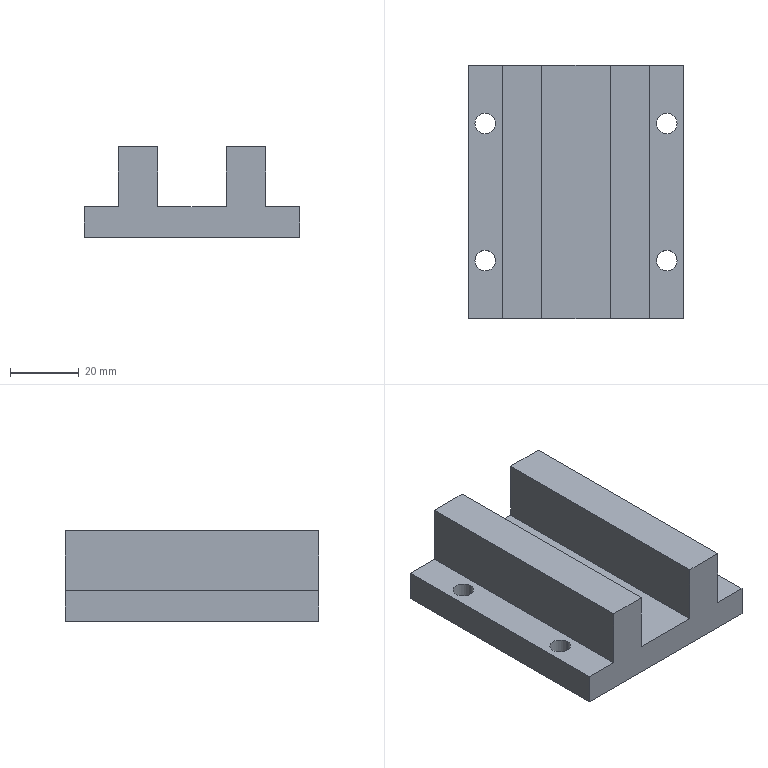Part | STEP file | Guide rail sliding pair | 1 solid | 22 faces | box 63 x 74 x 26.5 mm | volume 70725 mm3 | plane 14 | cylinder 8 | commonest cylinder face diameters 6 x8
STEP:
#1=CARTESIAN_POINT('',(9.179,-38.565,9.));
#2=VERTEX_POINT('',#1);
#3=CARTESIAN_POINT('',(3.179,-38.565,9.));
#4=VERTEX_POINT('',#3);
#5=CARTESIAN_POINT('',(6.179,-38.565,9.));
#6=DIRECTION('',(0.,0.,-1.));
#7=DIRECTION('',(-1.,0.,0.));
#8=AXIS2_PLACEMENT_3D('',#5,#6,#7);
#9=CIRCLE('',#8,3.);
#10=EDGE_CURVE('',#2,#4,#9,.T.);
#11=ORIENTED_EDGE('',*,*,#10,.F.);
#12=CARTESIAN_POINT('',(9.179,-38.565,0.));
#13=VERTEX_POINT('',#12);
#14=CARTESIAN_POINT('',(9.179,-38.565,9.));
#15=DIRECTION('',(0.,0.,-1.));
#16=VECTOR('',#15,1000.);
#17=LINE('',#14,#16);
#18=EDGE_CURVE('',#2,#13,#17,.T.);
#19=ORIENTED_EDGE('',*,*,#18,.T.);
#20=CARTESIAN_POINT('',(3.179,-38.565,0.));
#21=VERTEX_POINT('',#20);
#22=CARTESIAN_POINT('',(6.179,-38.565,0.));
#23=DIRECTION('',(0.,0.,-1.));
#24=DIRECTION('',(-1.,0.,0.));
#25=AXIS2_PLACEMENT_3D('',#22,#23,#24);
#26=CIRCLE('',#25,3.);
#27=EDGE_CURVE('',#13,#21,#26,.T.);
#28=ORIENTED_EDGE('',*,*,#27,.T.);
#29=CARTESIAN_POINT('',(3.179,-38.565,9.));
#30=DIRECTION('',(0.,0.,-1.));
#31=VECTOR('',#30,1000.);
#32=LINE('',#29,#31);
#33=EDGE_CURVE('',#4,#21,#32,.T.);
#34=ORIENTED_EDGE('',*,*,#33,.F.);
#35=EDGE_LOOP('',(#11,#19,#28,#34));
#36=FACE_OUTER_BOUND('',#35,.T.);
#37=CARTESIAN_POINT('',(6.179,-38.565,9.));
#38=DIRECTION('',(0.,0.,-1.));
#39=DIRECTION('',(-1.,0.,0.));
#40=AXIS2_PLACEMENT_3D('',#37,#38,#39);
#41=CYLINDRICAL_SURFACE('',#40,3.);
#42=ADVANCED_FACE('',(#36),#41,.F.);
#43=CARTESIAN_POINT('',(9.179,1.435,9.));
#44=VERTEX_POINT('',#43);
#45=CARTESIAN_POINT('',(3.179,1.435,9.));
#46=VERTEX_POINT('',#45);
#47=CARTESIAN_POINT('',(6.179,1.435,9.));
#48=DIRECTION('',(0.,0.,-1.));
#49=DIRECTION('',(-1.,0.,0.));
#50=AXIS2_PLACEMENT_3D('',#47,#48,#49);
#51=CIRCLE('',#50,3.);
#52=EDGE_CURVE('',#44,#46,#51,.T.);
#53=ORIENTED_EDGE('',*,*,#52,.F.);
#54=CARTESIAN_POINT('',(9.179,1.435,0.));
#55=VERTEX_POINT('',#54);
#56=CARTESIAN_POINT('',(9.179,1.435,9.));
#57=DIRECTION('',(0.,0.,-1.));
#58=VECTOR('',#57,1000.);
#59=LINE('',#56,#58);
#60=EDGE_CURVE('',#44,#55,#59,.T.);
#61=ORIENTED_EDGE('',*,*,#60,.T.);
#62=CARTESIAN_POINT('',(3.179,1.435,0.));
#63=VERTEX_POINT('',#62);
#64=CARTESIAN_POINT('',(6.179,1.435,0.));
#65=DIRECTION('',(0.,0.,-1.));
#66=DIRECTION('',(-1.,0.,0.));
#67=AXIS2_PLACEMENT_3D('',#64,#65,#66);
#68=CIRCLE('',#67,3.);
#69=EDGE_CURVE('',#55,#63,#68,.T.);
#70=ORIENTED_EDGE('',*,*,#69,.T.);
#71=CARTESIAN_POINT('',(3.179,1.435,9.));
#72=DIRECTION('',(0.,0.,-1.));
#73=VECTOR('',#72,1000.);
#74=LINE('',#71,#73);
#75=EDGE_CURVE('',#46,#63,#74,.T.);
#76=ORIENTED_EDGE('',*,*,#75,.F.);
#77=EDGE_LOOP('',(#53,#61,#70,#76));
#78=FACE_OUTER_BOUND('',#77,.T.);
#79=CARTESIAN_POINT('',(6.179,1.435,9.));
#80=DIRECTION('',(0.,0.,-1.));
#81=DIRECTION('',(-1.,0.,0.));
#82=AXIS2_PLACEMENT_3D('',#79,#80,#81);
#83=CYLINDRICAL_SURFACE('',#82,3.);
#84=ADVANCED_FACE('',(#78),#83,.F.);
#85=CARTESIAN_POINT('',(-43.821,1.435,9.));
#86=VERTEX_POINT('',#85);
#87=CARTESIAN_POINT('',(-49.821,1.435,9.));
#88=VERTEX_POINT('',#87);
#89=CARTESIAN_POINT('',(-46.821,1.435,9.));
#90=DIRECTION('',(0.,0.,-1.));
#91=DIRECTION('',(-1.,0.,0.));
#92=AXIS2_PLACEMENT_3D('',#89,#90,#91);
#93=CIRCLE('',#92,3.);
#94=EDGE_CURVE('',#86,#88,#93,.T.);
#95=ORIENTED_EDGE('',*,*,#94,.F.);
#96=CARTESIAN_POINT('',(-43.821,1.435,0.));
#97=VERTEX_POINT('',#96);
#98=CARTESIAN_POINT('',(-43.821,1.435,9.));
#99=DIRECTION('',(0.,0.,-1.));
#100=VECTOR('',#99,1000.);
#101=LINE('',#98,#100);
#102=EDGE_CURVE('',#86,#97,#101,.T.);
#103=ORIENTED_EDGE('',*,*,#102,.T.);
#104=CARTESIAN_POINT('',(-49.821,1.435,0.));
#105=VERTEX_POINT('',#104);
#106=CARTESIAN_POINT('',(-46.821,1.435,0.));
#107=DIRECTION('',(0.,0.,-1.));
#108=DIRECTION('',(-1.,0.,0.));
#109=AXIS2_PLACEMENT_3D('',#106,#107,#108);
#110=CIRCLE('',#109,3.);
#111=EDGE_CURVE('',#97,#105,#110,.T.);
#112=ORIENTED_EDGE('',*,*,#111,.T.);
#113=CARTESIAN_POINT('',(-49.821,1.435,9.));
#114=DIRECTION('',(0.,0.,-1.));
#115=VECTOR('',#114,1000.);
#116=LINE('',#113,#115);
#117=EDGE_CURVE('',#88,#105,#116,.T.);
#118=ORIENTED_EDGE('',*,*,#117,.F.);
#119=EDGE_LOOP('',(#95,#103,#112,#118));
#120=FACE_OUTER_BOUND('',#119,.T.);
#121=CARTESIAN_POINT('',(-46.821,1.435,9.));
#122=DIRECTION('',(0.,0.,-1.));
#123=DIRECTION('',(-1.,0.,0.));
#124=AXIS2_PLACEMENT_3D('',#121,#122,#123);
#125=CYLINDRICAL_SURFACE('',#124,3.);
#126=ADVANCED_FACE('',(#120),#125,.F.);
#127=CARTESIAN_POINT('',(-43.821,-38.565,9.));
#128=VERTEX_POINT('',#127);
#129=CARTESIAN_POINT('',(-49.821,-38.565,9.));
#130=VERTEX_POINT('',#129);
#131=CARTESIAN_POINT('',(-46.821,-38.565,9.));
#132=DIRECTION('',(0.,0.,-1.));
#133=DIRECTION('',(-1.,0.,0.));
#134=AXIS2_PLACEMENT_3D('',#131,#132,#133);
#135=CIRCLE('',#134,3.);
#136=EDGE_CURVE('',#128,#130,#135,.T.);
#137=ORIENTED_EDGE('',*,*,#136,.F.);
#138=CARTESIAN_POINT('',(-43.821,-38.565,0.));
#139=VERTEX_POINT('',#138);
#140=CARTESIAN_POINT('',(-43.821,-38.565,9.));
#141=DIRECTION('',(0.,0.,-1.));
#142=VECTOR('',#141,1000.);
#143=LINE('',#140,#142);
#144=EDGE_CURVE('',#128,#139,#143,.T.);
#145=ORIENTED_EDGE('',*,*,#144,.T.);
#146=CARTESIAN_POINT('',(-49.821,-38.565,0.));
#147=VERTEX_POINT('',#146);
#148=CARTESIAN_POINT('',(-46.821,-38.565,0.));
#149=DIRECTION('',(0.,0.,-1.));
#150=DIRECTION('',(-1.,0.,0.));
#151=AXIS2_PLACEMENT_3D('',#148,#149,#150);
#152=CIRCLE('',#151,3.);
#153=EDGE_CURVE('',#139,#147,#152,.T.);
#154=ORIENTED_EDGE('',*,*,#153,.T.);
#155=CARTESIAN_POINT('',(-49.821,-38.565,9.));
#156=DIRECTION('',(0.,0.,-1.));
#157=VECTOR('',#156,1000.);
#158=LINE('',#155,#157);
#159=EDGE_CURVE('',#130,#147,#158,.T.);
#160=ORIENTED_EDGE('',*,*,#159,.F.);
#161=EDGE_LOOP('',(#137,#145,#154,#160));
#162=FACE_OUTER_BOUND('',#161,.T.);
#163=CARTESIAN_POINT('',(-46.821,-38.565,9.));
#164=DIRECTION('',(0.,0.,-1.));
#165=DIRECTION('',(-1.,0.,0.));
#166=AXIS2_PLACEMENT_3D('',#163,#164,#165);
#167=CYLINDRICAL_SURFACE('',#166,3.);
#168=ADVANCED_FACE('',(#162),#167,.F.);
#169=CARTESIAN_POINT('',(6.179,-38.565,0.));
#170=DIRECTION('',(0.,0.,-1.));
#171=DIRECTION('',(-1.,0.,0.));
#172=AXIS2_PLACEMENT_3D('',#169,#170,#171);
#173=CIRCLE('',#172,3.);
#174=EDGE_CURVE('',#21,#13,#173,.T.);
#175=ORIENTED_EDGE('',*,*,#174,.F.);
#176=ORIENTED_EDGE('',*,*,#27,.F.);
#177=EDGE_LOOP('',(#175,#176));
#178=FACE_BOUND('',#177,.T.);
#179=CARTESIAN_POINT('',(6.179,1.435,0.));
#180=DIRECTION('',(0.,0.,-1.));
#181=DIRECTION('',(-1.,0.,0.));
#182=AXIS2_PLACEMENT_3D('',#179,#180,#181);
#183=CIRCLE('',#182,3.);
#184=EDGE_CURVE('',#63,#55,#183,.T.);
#185=ORIENTED_EDGE('',*,*,#184,.F.);
#186=ORIENTED_EDGE('',*,*,#69,.F.);
#187=EDGE_LOOP('',(#185,#186));
#188=FACE_BOUND('',#187,.T.);
#189=CARTESIAN_POINT('',(11.179,18.435,0.));
#190=VERTEX_POINT('',#189);
#191=CARTESIAN_POINT('',(-51.821,18.435,0.));
#192=VERTEX_POINT('',#191);
#193=CARTESIAN_POINT('',(-51.821,18.435,0.));
#194=DIRECTION('',(-1.,0.,0.));
#195=VECTOR('',#194,1000.);
#196=LINE('',#193,#195);
#197=EDGE_CURVE('',#190,#192,#196,.T.);
#198=ORIENTED_EDGE('',*,*,#197,.F.);
#199=CARTESIAN_POINT('',(11.179,-55.565,0.));
#200=VERTEX_POINT('',#199);
#201=CARTESIAN_POINT('',(11.179,-55.565,0.));
#202=DIRECTION('',(0.,1.,0.));
#203=VECTOR('',#202,1000.);
#204=LINE('',#201,#203);
#205=EDGE_CURVE('',#200,#190,#204,.T.);
#206=ORIENTED_EDGE('',*,*,#205,.F.);
#207=CARTESIAN_POINT('',(-51.821,-55.565,0.));
#208=VERTEX_POINT('',#207);
#209=CARTESIAN_POINT('',(-51.821,-55.565,0.));
#210=DIRECTION('',(1.,0.,0.));
#211=VECTOR('',#210,1000.);
#212=LINE('',#209,#211);
#213=EDGE_CURVE('',#208,#200,#212,.T.);
#214=ORIENTED_EDGE('',*,*,#213,.F.);
#215=CARTESIAN_POINT('',(-51.821,-55.565,0.));
#216=DIRECTION('',(0.,-1.,0.));
#217=VECTOR('',#216,1000.);
#218=LINE('',#215,#217);
#219=EDGE_CURVE('',#192,#208,#218,.T.);
#220=ORIENTED_EDGE('',*,*,#219,.F.);
#221=EDGE_LOOP('',(#198,#206,#214,#220));
#222=FACE_OUTER_BOUND('',#221,.T.);
#223=CARTESIAN_POINT('',(-46.821,1.435,0.));
#224=DIRECTION('',(0.,0.,-1.));
#225=DIRECTION('',(-1.,0.,0.));
#226=AXIS2_PLACEMENT_3D('',#223,#224,#225);
#227=CIRCLE('',#226,3.);
#228=EDGE_CURVE('',#105,#97,#227,.T.);
#229=ORIENTED_EDGE('',*,*,#228,.F.);
#230=ORIENTED_EDGE('',*,*,#111,.F.);
#231=EDGE_LOOP('',(#229,#230));
#232=FACE_BOUND('',#231,.T.);
#233=CARTESIAN_POINT('',(-46.821,-38.565,0.));
#234=DIRECTION('',(0.,0.,-1.));
#235=DIRECTION('',(-1.,0.,0.));
#236=AXIS2_PLACEMENT_3D('',#233,#234,#235);
#237=CIRCLE('',#236,3.);
#238=EDGE_CURVE('',#147,#139,#237,.T.);
#239=ORIENTED_EDGE('',*,*,#238,.F.);
#240=ORIENTED_EDGE('',*,*,#153,.F.);
#241=EDGE_LOOP('',(#239,#240));
#242=FACE_BOUND('',#241,.T.);
#243=CARTESIAN_POINT('',(-51.821,-55.565,0.));
#244=DIRECTION('',(0.,0.,1.));
#245=DIRECTION('',(1.,0.,0.));
#246=AXIS2_PLACEMENT_3D('',#243,#244,#245);
#247=PLANE('',#246);
#248=ADVANCED_FACE('',(#178,#188,#222,#232,#242),#247,.F.);
#249=ORIENTED_EDGE('',*,*,#18,.F.);
#250=CARTESIAN_POINT('',(6.179,-38.565,9.));
#251=DIRECTION('',(0.,0.,-1.));
#252=DIRECTION('',(-1.,0.,0.));
#253=AXIS2_PLACEMENT_3D('',#250,#251,#252);
#254=CIRCLE('',#253,3.);
#255=EDGE_CURVE('',#4,#2,#254,.T.);
#256=ORIENTED_EDGE('',*,*,#255,.F.);
#257=ORIENTED_EDGE('',*,*,#33,.T.);
#258=ORIENTED_EDGE('',*,*,#174,.T.);
#259=EDGE_LOOP('',(#249,#256,#257,#258));
#260=FACE_OUTER_BOUND('',#259,.T.);
#261=CARTESIAN_POINT('',(6.179,-38.565,9.));
#262=DIRECTION('',(0.,0.,-1.));
#263=DIRECTION('',(-1.,0.,0.));
#264=AXIS2_PLACEMENT_3D('',#261,#262,#263);
#265=CYLINDRICAL_SURFACE('',#264,3.);
#266=ADVANCED_FACE('',(#260),#265,.F.);
#267=ORIENTED_EDGE('',*,*,#60,.F.);
#268=CARTESIAN_POINT('',(6.179,1.435,9.));
#269=DIRECTION('',(0.,0.,-1.));
#270=DIRECTION('',(-1.,0.,0.));
#271=AXIS2_PLACEMENT_3D('',#268,#269,#270);
#272=CIRCLE('',#271,3.);
#273=EDGE_CURVE('',#46,#44,#272,.T.);
#274=ORIENTED_EDGE('',*,*,#273,.F.);
#275=ORIENTED_EDGE('',*,*,#75,.T.);
#276=ORIENTED_EDGE('',*,*,#184,.T.);
#277=EDGE_LOOP('',(#267,#274,#275,#276));
#278=FACE_OUTER_BOUND('',#277,.T.);
#279=CARTESIAN_POINT('',(6.179,1.435,9.));
#280=DIRECTION('',(0.,0.,-1.));
#281=DIRECTION('',(-1.,0.,0.));
#282=AXIS2_PLACEMENT_3D('',#279,#280,#281);
#283=CYLINDRICAL_SURFACE('',#282,3.);
#284=ADVANCED_FACE('',(#278),#283,.F.);
#285=CARTESIAN_POINT('',(-51.821,-55.565,9.));
#286=VERTEX_POINT('',#285);
#287=CARTESIAN_POINT('',(-51.821,-55.565,9.));
#288=DIRECTION('',(0.,0.,-1.));
#289=VECTOR('',#288,1000.);
#290=LINE('',#287,#289);
#291=EDGE_CURVE('',#286,#208,#290,.T.);
#292=ORIENTED_EDGE('',*,*,#291,.F.);
#293=CARTESIAN_POINT('',(-51.821,18.435,9.));
#294=VERTEX_POINT('',#293);
#295=CARTESIAN_POINT('',(-51.821,18.435,9.));
#296=DIRECTION('',(0.,-1.,0.));
#297=VECTOR('',#296,1000.);
#298=LINE('',#295,#297);
#299=EDGE_CURVE('',#294,#286,#298,.T.);
#300=ORIENTED_EDGE('',*,*,#299,.F.);
#301=CARTESIAN_POINT('',(-51.821,18.435,9.));
#302=DIRECTION('',(0.,0.,1.));
#303=VECTOR('',#302,1000.);
#304=LINE('',#301,#303);
#305=EDGE_CURVE('',#192,#294,#304,.T.);
#306=ORIENTED_EDGE('',*,*,#305,.F.);
#307=ORIENTED_EDGE('',*,*,#219,.T.);
#308=EDGE_LOOP('',(#292,#300,#306,#307));
#309=FACE_OUTER_BOUND('',#308,.T.);
#310=CARTESIAN_POINT('',(-51.821,18.435,9.));
#311=DIRECTION('',(1.,0.,0.));
#312=DIRECTION('',(0.,0.,-1.));
#313=AXIS2_PLACEMENT_3D('',#310,#311,#312);
#314=PLANE('',#313);
#315=ADVANCED_FACE('',(#309),#314,.F.);
#316=CARTESIAN_POINT('',(-30.321,18.435,9.));
#317=VERTEX_POINT('',#316);
#318=CARTESIAN_POINT('',(-30.321,18.435,26.5));
#319=VERTEX_POINT('',#318);
#320=CARTESIAN_POINT('',(-30.321,18.435,9.));
#321=DIRECTION('',(0.,0.,1.));
#322=VECTOR('',#321,1000.);
#323=LINE('',#320,#322);
#324=EDGE_CURVE('',#317,#319,#323,.T.);
#325=ORIENTED_EDGE('',*,*,#324,.F.);
#326=CARTESIAN_POINT('',(-10.321,18.435,9.));
#327=VERTEX_POINT('',#326);
#328=CARTESIAN_POINT('',(-51.821,18.435,9.));
#329=DIRECTION('',(-1.,0.,0.));
#330=VECTOR('',#329,1000.);
#331=LINE('',#328,#330);
#332=EDGE_CURVE('',#327,#317,#331,.T.);
#333=ORIENTED_EDGE('',*,*,#332,.F.);
#334=CARTESIAN_POINT('',(-10.321,18.435,26.5));
#335=VERTEX_POINT('',#334);
#336=CARTESIAN_POINT('',(-10.321,18.435,9.));
#337=DIRECTION('',(0.,0.,-1.));
#338=VECTOR('',#337,1000.);
#339=LINE('',#336,#338);
#340=EDGE_CURVE('',#335,#327,#339,.T.);
#341=ORIENTED_EDGE('',*,*,#340,.F.);
#342=CARTESIAN_POINT('',(1.179,18.435,26.5));
#343=VERTEX_POINT('',#342);
#344=CARTESIAN_POINT('',(-51.821,18.435,26.5));
#345=DIRECTION('',(-1.,0.,0.));
#346=VECTOR('',#345,1000.);
#347=LINE('',#344,#346);
#348=EDGE_CURVE('',#343,#335,#347,.T.);
#349=ORIENTED_EDGE('',*,*,#348,.F.);
#350=CARTESIAN_POINT('',(1.179,18.435,9.));
#351=VERTEX_POINT('',#350);
#352=CARTESIAN_POINT('',(1.179,18.435,9.));
#353=DIRECTION('',(0.,0.,1.));
#354=VECTOR('',#353,1000.);
#355=LINE('',#352,#354);
#356=EDGE_CURVE('',#351,#343,#355,.T.);
#357=ORIENTED_EDGE('',*,*,#356,.F.);
#358=CARTESIAN_POINT('',(11.179,18.435,9.));
#359=VERTEX_POINT('',#358);
#360=CARTESIAN_POINT('',(-51.821,18.435,9.));
#361=DIRECTION('',(-1.,0.,0.));
#362=VECTOR('',#361,1000.);
#363=LINE('',#360,#362);
#364=EDGE_CURVE('',#359,#351,#363,.T.);
#365=ORIENTED_EDGE('',*,*,#364,.F.);
#366=CARTESIAN_POINT('',(11.179,18.435,9.));
#367=DIRECTION('',(0.,0.,1.));
#368=VECTOR('',#367,1000.);
#369=LINE('',#366,#368);
#370=EDGE_CURVE('',#190,#359,#369,.T.);
#371=ORIENTED_EDGE('',*,*,#370,.F.);
#372=ORIENTED_EDGE('',*,*,#197,.T.);
#373=ORIENTED_EDGE('',*,*,#305,.T.);
#374=CARTESIAN_POINT('',(-41.821,18.435,9.));
#375=VERTEX_POINT('',#374);
#376=CARTESIAN_POINT('',(-51.821,18.435,9.));
#377=DIRECTION('',(-1.,0.,0.));
#378=VECTOR('',#377,1000.);
#379=LINE('',#376,#378);
#380=EDGE_CURVE('',#375,#294,#379,.T.);
#381=ORIENTED_EDGE('',*,*,#380,.F.);
#382=CARTESIAN_POINT('',(-41.821,18.435,26.5));
#383=VERTEX_POINT('',#382);
#384=CARTESIAN_POINT('',(-41.821,18.435,9.));
#385=DIRECTION('',(0.,0.,-1.));
#386=VECTOR('',#385,1000.);
#387=LINE('',#384,#386);
#388=EDGE_CURVE('',#383,#375,#387,.T.);
#389=ORIENTED_EDGE('',*,*,#388,.F.);
#390=CARTESIAN_POINT('',(-51.821,18.435,26.5));
#391=DIRECTION('',(-1.,0.,0.));
#392=VECTOR('',#391,1000.);
#393=LINE('',#390,#392);
#394=EDGE_CURVE('',#319,#383,#393,.T.);
#395=ORIENTED_EDGE('',*,*,#394,.F.);
#396=EDGE_LOOP('',(#325,#333,#341,#349,#357,#365,#371,#372,#373,#381,#389,#395));
#397=FACE_OUTER_BOUND('',#396,.T.);
#398=CARTESIAN_POINT('',(-51.821,18.435,9.));
#399=DIRECTION('',(0.,-1.,0.));
#400=DIRECTION('',(0.,0.,-1.));
#401=AXIS2_PLACEMENT_3D('',#398,#399,#400);
#402=PLANE('',#401);
#403=ADVANCED_FACE('',(#397),#402,.F.);
#404=ORIENTED_EDGE('',*,*,#370,.T.);
#405=CARTESIAN_POINT('',(11.179,-55.565,9.));
#406=VERTEX_POINT('',#405);
#407=CARTESIAN_POINT('',(11.179,18.435,9.));
#408=DIRECTION('',(0.,1.,0.));
#409=VECTOR('',#408,1000.);
#410=LINE('',#407,#409);
#411=EDGE_CURVE('',#406,#359,#410,.T.);
#412=ORIENTED_EDGE('',*,*,#411,.F.);
#413=CARTESIAN_POINT('',(11.179,-55.565,9.));
#414=DIRECTION('',(0.,0.,1.));
#415=VECTOR('',#414,1000.);
#416=LINE('',#413,#415);
#417=EDGE_CURVE('',#200,#406,#416,.T.);
#418=ORIENTED_EDGE('',*,*,#417,.F.);
#419=ORIENTED_EDGE('',*,*,#205,.T.);
#420=EDGE_LOOP('',(#404,#412,#418,#419));
#421=FACE_OUTER_BOUND('',#420,.T.);
#422=CARTESIAN_POINT('',(11.179,18.435,9.));
#423=DIRECTION('',(-1.,0.,0.));
#424=DIRECTION('',(0.,0.,1.));
#425=AXIS2_PLACEMENT_3D('',#422,#423,#424);
#426=PLANE('',#425);
#427=ADVANCED_FACE('',(#421),#426,.F.);
#428=CARTESIAN_POINT('',(-30.321,-55.565,26.5));
#429=VERTEX_POINT('',#428);
#430=CARTESIAN_POINT('',(-30.321,-55.565,9.));
#431=VERTEX_POINT('',#430);
#432=CARTESIAN_POINT('',(-30.321,-55.565,9.));
#433=DIRECTION('',(0.,0.,-1.));
#434=VECTOR('',#433,1000.);
#435=LINE('',#432,#434);
#436=EDGE_CURVE('',#429,#431,#435,.T.);
#437=ORIENTED_EDGE('',*,*,#436,.F.);
#438=CARTESIAN_POINT('',(-41.821,-55.565,26.5));
#439=VERTEX_POINT('',#438);
#440=CARTESIAN_POINT('',(-51.821,-55.565,26.5));
#441=DIRECTION('',(1.,0.,0.));
#442=VECTOR('',#441,1000.);
#443=LINE('',#440,#442);
#444=EDGE_CURVE('',#439,#429,#443,.T.);
#445=ORIENTED_EDGE('',*,*,#444,.F.);
#446=CARTESIAN_POINT('',(-41.821,-55.565,9.));
#447=VERTEX_POINT('',#446);
#448=CARTESIAN_POINT('',(-41.821,-55.565,9.));
#449=DIRECTION('',(0.,0.,1.));
#450=VECTOR('',#449,1000.);
#451=LINE('',#448,#450);
#452=EDGE_CURVE('',#447,#439,#451,.T.);
#453=ORIENTED_EDGE('',*,*,#452,.F.);
#454=CARTESIAN_POINT('',(-51.821,-55.565,9.));
#455=DIRECTION('',(1.,0.,0.));
#456=VECTOR('',#455,1000.);
#457=LINE('',#454,#456);
#458=EDGE_CURVE('',#286,#447,#457,.T.);
#459=ORIENTED_EDGE('',*,*,#458,.F.);
#460=ORIENTED_EDGE('',*,*,#291,.T.);
#461=ORIENTED_EDGE('',*,*,#213,.T.);
#462=ORIENTED_EDGE('',*,*,#417,.T.);
#463=CARTESIAN_POINT('',(1.179,-55.565,9.));
#464=VERTEX_POINT('',#463);
#465=CARTESIAN_POINT('',(-51.821,-55.565,9.));
#466=DIRECTION('',(1.,0.,0.));
#467=VECTOR('',#466,1000.);
#468=LINE('',#465,#467);
#469=EDGE_CURVE('',#464,#406,#468,.T.);
#470=ORIENTED_EDGE('',*,*,#469,.F.);
#471=CARTESIAN_POINT('',(1.179,-55.565,26.5));
#472=VERTEX_POINT('',#471);
#473=CARTESIAN_POINT('',(1.179,-55.565,9.));
#474=DIRECTION('',(0.,0.,-1.));
#475=VECTOR('',#474,1000.);
#476=LINE('',#473,#475);
#477=EDGE_CURVE('',#472,#464,#476,.T.);
#478=ORIENTED_EDGE('',*,*,#477,.F.);
#479=CARTESIAN_POINT('',(-10.321,-55.565,26.5));
#480=VERTEX_POINT('',#479);
#481=CARTESIAN_POINT('',(-51.821,-55.565,26.5));
#482=DIRECTION('',(1.,0.,0.));
#483=VECTOR('',#482,1000.);
#484=LINE('',#481,#483);
#485=EDGE_CURVE('',#480,#472,#484,.T.);
#486=ORIENTED_EDGE('',*,*,#485,.F.);
#487=CARTESIAN_POINT('',(-10.321,-55.565,9.));
#488=VERTEX_POINT('',#487);
#489=CARTESIAN_POINT('',(-10.321,-55.565,9.));
#490=DIRECTION('',(0.,0.,1.));
#491=VECTOR('',#490,1000.);
#492=LINE('',#489,#491);
#493=EDGE_CURVE('',#488,#480,#492,.T.);
#494=ORIENTED_EDGE('',*,*,#493,.F.);
#495=CARTESIAN_POINT('',(-51.821,-55.565,9.));
#496=DIRECTION('',(1.,0.,0.));
#497=VECTOR('',#496,1000.);
#498=LINE('',#495,#497);
#499=EDGE_CURVE('',#431,#488,#498,.T.);
#500=ORIENTED_EDGE('',*,*,#499,.F.);
#501=EDGE_LOOP('',(#437,#445,#453,#459,#460,#461,#462,#470,#478,#486,#494,#500));
#502=FACE_OUTER_BOUND('',#501,.T.);
#503=CARTESIAN_POINT('',(-51.821,-55.565,9.));
#504=DIRECTION('',(0.,1.,0.));
#505=DIRECTION('',(0.,0.,1.));
#506=AXIS2_PLACEMENT_3D('',#503,#504,#505);
#507=PLANE('',#506);
#508=ADVANCED_FACE('',(#502),#507,.F.);
#509=ORIENTED_EDGE('',*,*,#102,.F.);
#510=CARTESIAN_POINT('',(-46.821,1.435,9.));
#511=DIRECTION('',(0.,0.,-1.));
#512=DIRECTION('',(-1.,0.,0.));
#513=AXIS2_PLACEMENT_3D('',#510,#511,#512);
#514=CIRCLE('',#513,3.);
#515=EDGE_CURVE('',#88,#86,#514,.T.);
#516=ORIENTED_EDGE('',*,*,#515,.F.);
#517=ORIENTED_EDGE('',*,*,#117,.T.);
#518=ORIENTED_EDGE('',*,*,#228,.T.);
#519=EDGE_LOOP('',(#509,#516,#517,#518));
#520=FACE_OUTER_BOUND('',#519,.T.);
#521=CARTESIAN_POINT('',(-46.821,1.435,9.));
#522=DIRECTION('',(0.,0.,-1.));
#523=DIRECTION('',(-1.,0.,0.));
#524=AXIS2_PLACEMENT_3D('',#521,#522,#523);
#525=CYLINDRICAL_SURFACE('',#524,3.);
#526=ADVANCED_FACE('',(#520),#525,.F.);
#527=ORIENTED_EDGE('',*,*,#144,.F.);
#528=CARTESIAN_POINT('',(-46.821,-38.565,9.));
#529=DIRECTION('',(0.,0.,-1.));
#530=DIRECTION('',(-1.,0.,0.));
#531=AXIS2_PLACEMENT_3D('',#528,#529,#530);
#532=CIRCLE('',#531,3.);
#533=EDGE_CURVE('',#130,#128,#532,.T.);
#534=ORIENTED_EDGE('',*,*,#533,.F.);
#535=ORIENTED_EDGE('',*,*,#159,.T.);
#536=ORIENTED_EDGE('',*,*,#238,.T.);
#537=EDGE_LOOP('',(#527,#534,#535,#536));
#538=FACE_OUTER_BOUND('',#537,.T.);
#539=CARTESIAN_POINT('',(-46.821,-38.565,9.));
#540=DIRECTION('',(0.,0.,-1.));
#541=DIRECTION('',(-1.,0.,0.));
#542=AXIS2_PLACEMENT_3D('',#539,#540,#541);
#543=CYLINDRICAL_SURFACE('',#542,3.);
#544=ADVANCED_FACE('',(#538),#543,.F.);
#545=ORIENTED_EDGE('',*,*,#255,.T.);
#546=ORIENTED_EDGE('',*,*,#10,.T.);
#547=EDGE_LOOP('',(#545,#546));
#548=FACE_BOUND('',#547,.T.);
#549=ORIENTED_EDGE('',*,*,#273,.T.);
#550=ORIENTED_EDGE('',*,*,#52,.T.);
#551=EDGE_LOOP('',(#549,#550));
#552=FACE_BOUND('',#551,.T.);
#553=ORIENTED_EDGE('',*,*,#411,.T.);
#554=ORIENTED_EDGE('',*,*,#364,.T.);
#555=CARTESIAN_POINT('',(1.179,-55.565,9.));
#556=DIRECTION('',(0.,-1.,0.));
#557=VECTOR('',#556,1000.);
#558=LINE('',#555,#557);
#559=EDGE_CURVE('',#351,#464,#558,.T.);
#560=ORIENTED_EDGE('',*,*,#559,.T.);
#561=ORIENTED_EDGE('',*,*,#469,.T.);
#562=EDGE_LOOP('',(#553,#554,#560,#561));
#563=FACE_OUTER_BOUND('',#562,.T.);
#564=CARTESIAN_POINT('',(-51.821,-55.565,9.));
#565=DIRECTION('',(0.,0.,1.));
#566=DIRECTION('',(1.,0.,0.));
#567=AXIS2_PLACEMENT_3D('',#564,#565,#566);
#568=PLANE('',#567);
#569=ADVANCED_FACE('',(#548,#552,#563),#568,.T.);
#570=ORIENTED_EDGE('',*,*,#533,.T.);
#571=ORIENTED_EDGE('',*,*,#136,.T.);
#572=EDGE_LOOP('',(#570,#571));
#573=FACE_BOUND('',#572,.T.);
#574=ORIENTED_EDGE('',*,*,#515,.T.);
#575=ORIENTED_EDGE('',*,*,#94,.T.);
#576=EDGE_LOOP('',(#574,#575));
#577=FACE_BOUND('',#576,.T.);
#578=ORIENTED_EDGE('',*,*,#299,.T.);
#579=ORIENTED_EDGE('',*,*,#458,.T.);
#580=CARTESIAN_POINT('',(-41.821,-55.565,9.));
#581=DIRECTION('',(0.,1.,0.));
#582=VECTOR('',#581,1000.);
#583=LINE('',#580,#582);
#584=EDGE_CURVE('',#447,#375,#583,.T.);
#585=ORIENTED_EDGE('',*,*,#584,.T.);
#586=ORIENTED_EDGE('',*,*,#380,.T.);
#587=EDGE_LOOP('',(#578,#579,#585,#586));
#588=FACE_OUTER_BOUND('',#587,.T.);
#589=CARTESIAN_POINT('',(-51.821,-55.565,9.));
#590=DIRECTION('',(0.,0.,1.));
#591=DIRECTION('',(1.,0.,0.));
#592=AXIS2_PLACEMENT_3D('',#589,#590,#591);
#593=PLANE('',#592);
#594=ADVANCED_FACE('',(#573,#577,#588),#593,.T.);
#595=CARTESIAN_POINT('',(-41.821,-55.565,26.5));
#596=DIRECTION('',(0.,-1.,0.));
#597=VECTOR('',#596,1000.);
#598=LINE('',#595,#597);
#599=EDGE_CURVE('',#383,#439,#598,.T.);
#600=ORIENTED_EDGE('',*,*,#599,.T.);
#601=ORIENTED_EDGE('',*,*,#444,.T.);
#602=CARTESIAN_POINT('',(-30.321,-55.565,26.5));
#603=DIRECTION('',(0.,1.,0.));
#604=VECTOR('',#603,1000.);
#605=LINE('',#602,#604);
#606=EDGE_CURVE('',#429,#319,#605,.T.);
#607=ORIENTED_EDGE('',*,*,#606,.T.);
#608=ORIENTED_EDGE('',*,*,#394,.T.);
#609=EDGE_LOOP('',(#600,#601,#607,#608));
#610=FACE_OUTER_BOUND('',#609,.T.);
#611=CARTESIAN_POINT('',(-41.821,-55.565,26.5));
#612=DIRECTION('',(0.,0.,1.));
#613=DIRECTION('',(1.,0.,0.));
#614=AXIS2_PLACEMENT_3D('',#611,#612,#613);
#615=PLANE('',#614);
#616=ADVANCED_FACE('',(#610),#615,.T.);
#617=ORIENTED_EDGE('',*,*,#436,.T.);
#618=CARTESIAN_POINT('',(-30.321,18.435,9.));
#619=DIRECTION('',(0.,-1.,0.));
#620=VECTOR('',#619,1000.);
#621=LINE('',#618,#620);
#622=EDGE_CURVE('',#317,#431,#621,.T.);
#623=ORIENTED_EDGE('',*,*,#622,.F.);
#624=ORIENTED_EDGE('',*,*,#324,.T.);
#625=ORIENTED_EDGE('',*,*,#606,.F.);
#626=EDGE_LOOP('',(#617,#623,#624,#625));
#627=FACE_OUTER_BOUND('',#626,.T.);
#628=CARTESIAN_POINT('',(-30.321,18.435,9.));
#629=DIRECTION('',(-1.,0.,0.));
#630=DIRECTION('',(0.,0.,1.));
#631=AXIS2_PLACEMENT_3D('',#628,#629,#630);
#632=PLANE('',#631);
#633=ADVANCED_FACE('',(#627),#632,.F.);
#634=CARTESIAN_POINT('',(-10.321,-55.565,9.));
#635=DIRECTION('',(0.,1.,0.));
#636=VECTOR('',#635,1000.);
#637=LINE('',#634,#636);
#638=EDGE_CURVE('',#488,#327,#637,.T.);
#639=ORIENTED_EDGE('',*,*,#638,.T.);
#640=ORIENTED_EDGE('',*,*,#332,.T.);
#641=ORIENTED_EDGE('',*,*,#622,.T.);
#642=ORIENTED_EDGE('',*,*,#499,.T.);
#643=EDGE_LOOP('',(#639,#640,#641,#642));
#644=FACE_OUTER_BOUND('',#643,.T.);
#645=CARTESIAN_POINT('',(-30.321,-55.565,9.));
#646=DIRECTION('',(0.,0.,1.));
#647=DIRECTION('',(1.,0.,0.));
#648=AXIS2_PLACEMENT_3D('',#645,#646,#647);
#649=PLANE('',#648);
#650=ADVANCED_FACE('',(#644),#649,.T.);
#651=ORIENTED_EDGE('',*,*,#340,.T.);
#652=ORIENTED_EDGE('',*,*,#638,.F.);
#653=ORIENTED_EDGE('',*,*,#493,.T.);
#654=CARTESIAN_POINT('',(-10.321,18.435,26.5));
#655=DIRECTION('',(0.,-1.,0.));
#656=VECTOR('',#655,1000.);
#657=LINE('',#654,#656);
#658=EDGE_CURVE('',#335,#480,#657,.T.);
#659=ORIENTED_EDGE('',*,*,#658,.F.);
#660=EDGE_LOOP('',(#651,#652,#653,#659));
#661=FACE_OUTER_BOUND('',#660,.T.);
#662=CARTESIAN_POINT('',(-10.321,18.435,9.));
#663=DIRECTION('',(1.,0.,0.));
#664=DIRECTION('',(0.,0.,-1.));
#665=AXIS2_PLACEMENT_3D('',#662,#663,#664);
#666=PLANE('',#665);
#667=ADVANCED_FACE('',(#661),#666,.F.);
#668=CARTESIAN_POINT('',(1.179,-55.565,26.5));
#669=DIRECTION('',(0.,1.,0.));
#670=VECTOR('',#669,1000.);
#671=LINE('',#668,#670);
#672=EDGE_CURVE('',#472,#343,#671,.T.);
#673=ORIENTED_EDGE('',*,*,#672,.T.);
#674=ORIENTED_EDGE('',*,*,#348,.T.);
#675=ORIENTED_EDGE('',*,*,#658,.T.);
#676=ORIENTED_EDGE('',*,*,#485,.T.);
#677=EDGE_LOOP('',(#673,#674,#675,#676));
#678=FACE_OUTER_BOUND('',#677,.T.);
#679=CARTESIAN_POINT('',(-41.821,-55.565,26.5));
#680=DIRECTION('',(0.,0.,1.));
#681=DIRECTION('',(1.,0.,0.));
#682=AXIS2_PLACEMENT_3D('',#679,#680,#681);
#683=PLANE('',#682);
#684=ADVANCED_FACE('',(#678),#683,.T.);
#685=ORIENTED_EDGE('',*,*,#356,.T.);
#686=ORIENTED_EDGE('',*,*,#672,.F.);
#687=ORIENTED_EDGE('',*,*,#477,.T.);
#688=ORIENTED_EDGE('',*,*,#559,.F.);
#689=EDGE_LOOP('',(#685,#686,#687,#688));
#690=FACE_OUTER_BOUND('',#689,.T.);
#691=CARTESIAN_POINT('',(1.179,18.435,26.5));
#692=DIRECTION('',(-1.,0.,0.));
#693=DIRECTION('',(0.,0.,1.));
#694=AXIS2_PLACEMENT_3D('',#691,#692,#693);
#695=PLANE('',#694);
#696=ADVANCED_FACE('',(#690),#695,.F.);
#697=ORIENTED_EDGE('',*,*,#452,.T.);
#698=ORIENTED_EDGE('',*,*,#599,.F.);
#699=ORIENTED_EDGE('',*,*,#388,.T.);
#700=ORIENTED_EDGE('',*,*,#584,.F.);
#701=EDGE_LOOP('',(#697,#698,#699,#700));
#702=FACE_OUTER_BOUND('',#701,.T.);
#703=CARTESIAN_POINT('',(-41.821,18.435,26.5));
#704=DIRECTION('',(1.,0.,0.));
#705=DIRECTION('',(0.,0.,-1.));
#706=AXIS2_PLACEMENT_3D('',#703,#704,#705);
#707=PLANE('',#706);
#708=ADVANCED_FACE('',(#702),#707,.F.);
#709=CLOSED_SHELL('',(#42,#84,#126,#168,#248,#266,#284,#315,#403,#427,#508,#526,#544,#569,#594,#616,#633,#650,#667,#684,#696,#708));
#710=MANIFOLD_SOLID_BREP('',#709);
#711=CARTESIAN_POINT('',(0.,0.,0.));
#712=DIRECTION('',(0.,0.,1.));
#713=DIRECTION('',(1.,0.,0.));
#714=AXIS2_PLACEMENT_3D('',#711,#712,#713);
#715=(LENGTH_UNIT()NAMED_UNIT(*)SI_UNIT(.MILLI.,.METRE.));
#716=UNCERTAINTY_MEASURE_WITH_UNIT(LENGTH_MEASURE(0.00001),#715,'','');
#717=(NAMED_UNIT(*)PLANE_ANGLE_UNIT()SI_UNIT($,.RADIAN.));
#718=(NAMED_UNIT(*)SI_UNIT($,.STERADIAN.)SOLID_ANGLE_UNIT());
#719=(GEOMETRIC_REPRESENTATION_CONTEXT(3)GLOBAL_UNCERTAINTY_ASSIGNED_CONTEXT((#716))GLOBAL_UNIT_ASSIGNED_CONTEXT((#715,#717,#718))REPRESENTATION_CONTEXT('',''));
#720=ADVANCED_BREP_SHAPE_REPRESENTATION('',(#710,#714),#719);